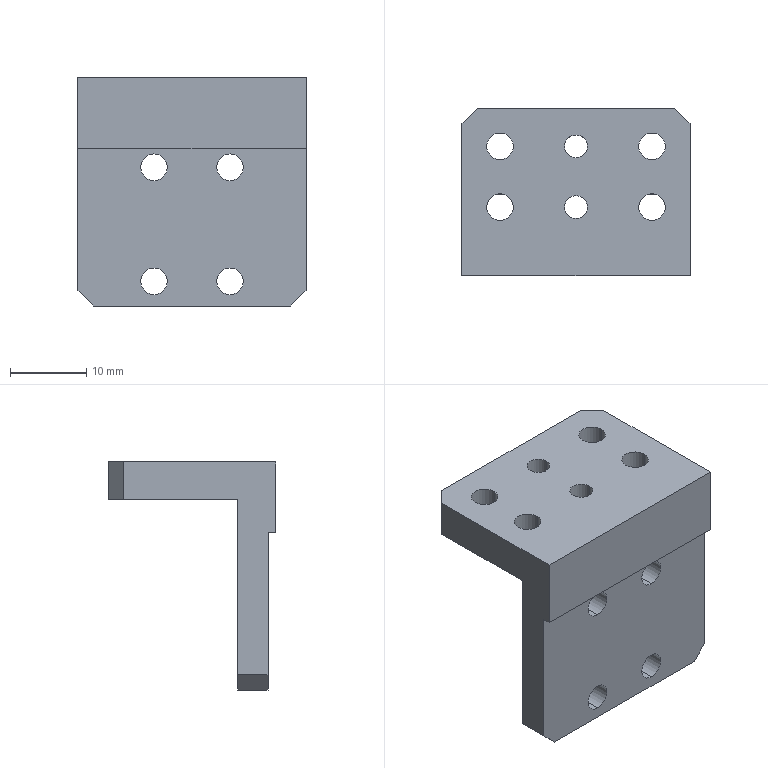Part | SolidWorks | features HoleWzd 3, ICE 2, Chamfer 1, Extrusion 1 | 1 solid | 34 faces | box 30 x 22 x 30 mm | volume 5974 mm3 | cylinder 20 | plane 14 | commonest cylinder face diameters 3.5 x16 3 x4
STEP:
#1=CARTESIAN_POINT('',(1.5,17.,15.));
#2=VERTEX_POINT('',#1);
#3=CARTESIAN_POINT('',(-1.5,17.,15.));
#4=VERTEX_POINT('',#3);
#5=CARTESIAN_POINT('',(0.,17.,15.));
#6=DIRECTION('',(0.,0.,-1.));
#7=DIRECTION('',(-1.,0.,0.));
#8=AXIS2_PLACEMENT_3D('',#5,#6,#7);
#9=CIRCLE('',#8,1.5);
#10=EDGE_CURVE('',#2,#4,#9,.T.);
#11=ORIENTED_EDGE('',*,*,#10,.F.);
#12=CARTESIAN_POINT('',(1.5,17.,10.));
#13=VERTEX_POINT('',#12);
#14=CARTESIAN_POINT('',(1.5,17.,10.));
#15=DIRECTION('',(0.,0.,-1.));
#16=VECTOR('',#15,1000.);
#17=LINE('',#14,#16);
#18=EDGE_CURVE('',#2,#13,#17,.T.);
#19=ORIENTED_EDGE('',*,*,#18,.T.);
#20=CARTESIAN_POINT('',(-1.5,17.,10.));
#21=VERTEX_POINT('',#20);
#22=CARTESIAN_POINT('',(0.,17.,10.));
#23=DIRECTION('',(0.,0.,-1.));
#24=DIRECTION('',(-1.,0.,0.));
#25=AXIS2_PLACEMENT_3D('',#22,#23,#24);
#26=CIRCLE('',#25,1.5);
#27=EDGE_CURVE('',#13,#21,#26,.T.);
#28=ORIENTED_EDGE('',*,*,#27,.T.);
#29=CARTESIAN_POINT('',(-1.5,17.,10.));
#30=DIRECTION('',(0.,0.,-1.));
#31=VECTOR('',#30,1000.);
#32=LINE('',#29,#31);
#33=EDGE_CURVE('',#4,#21,#32,.T.);
#34=ORIENTED_EDGE('',*,*,#33,.F.);
#35=EDGE_LOOP('',(#11,#19,#28,#34));
#36=FACE_OUTER_BOUND('',#35,.T.);
#37=CARTESIAN_POINT('',(0.,17.,10.));
#38=DIRECTION('',(0.,0.,-1.));
#39=DIRECTION('',(-1.,0.,0.));
#40=AXIS2_PLACEMENT_3D('',#37,#38,#39);
#41=CYLINDRICAL_SURFACE('',#40,1.5);
#42=ADVANCED_FACE('',(#36),#41,.F.);
#43=CARTESIAN_POINT('',(1.5,9.,15.));
#44=VERTEX_POINT('',#43);
#45=CARTESIAN_POINT('',(-1.5,9.,15.));
#46=VERTEX_POINT('',#45);
#47=CARTESIAN_POINT('',(0.,9.,15.));
#48=DIRECTION('',(0.,0.,-1.));
#49=DIRECTION('',(-1.,0.,0.));
#50=AXIS2_PLACEMENT_3D('',#47,#48,#49);
#51=CIRCLE('',#50,1.5);
#52=EDGE_CURVE('',#44,#46,#51,.T.);
#53=ORIENTED_EDGE('',*,*,#52,.F.);
#54=CARTESIAN_POINT('',(1.5,9.,10.));
#55=VERTEX_POINT('',#54);
#56=CARTESIAN_POINT('',(1.5,9.,10.));
#57=DIRECTION('',(0.,0.,-1.));
#58=VECTOR('',#57,1000.);
#59=LINE('',#56,#58);
#60=EDGE_CURVE('',#44,#55,#59,.T.);
#61=ORIENTED_EDGE('',*,*,#60,.T.);
#62=CARTESIAN_POINT('',(-1.5,9.,10.));
#63=VERTEX_POINT('',#62);
#64=CARTESIAN_POINT('',(0.,9.,10.));
#65=DIRECTION('',(0.,0.,-1.));
#66=DIRECTION('',(-1.,0.,0.));
#67=AXIS2_PLACEMENT_3D('',#64,#65,#66);
#68=CIRCLE('',#67,1.5);
#69=EDGE_CURVE('',#55,#63,#68,.T.);
#70=ORIENTED_EDGE('',*,*,#69,.T.);
#71=CARTESIAN_POINT('',(-1.5,9.,10.));
#72=DIRECTION('',(0.,0.,-1.));
#73=VECTOR('',#72,1000.);
#74=LINE('',#71,#73);
#75=EDGE_CURVE('',#46,#63,#74,.T.);
#76=ORIENTED_EDGE('',*,*,#75,.F.);
#77=EDGE_LOOP('',(#53,#61,#70,#76));
#78=FACE_OUTER_BOUND('',#77,.T.);
#79=CARTESIAN_POINT('',(0.,9.,10.));
#80=DIRECTION('',(0.,0.,-1.));
#81=DIRECTION('',(-1.,0.,0.));
#82=AXIS2_PLACEMENT_3D('',#79,#80,#81);
#83=CYLINDRICAL_SURFACE('',#82,1.5);
#84=ADVANCED_FACE('',(#78),#83,.F.);
#85=CARTESIAN_POINT('',(11.75,17.,15.));
#86=VERTEX_POINT('',#85);
#87=CARTESIAN_POINT('',(8.25,17.,15.));
#88=VERTEX_POINT('',#87);
#89=CARTESIAN_POINT('',(10.,17.,15.));
#90=DIRECTION('',(0.,0.,-1.));
#91=DIRECTION('',(-1.,0.,0.));
#92=AXIS2_PLACEMENT_3D('',#89,#90,#91);
#93=CIRCLE('',#92,1.75);
#94=EDGE_CURVE('',#86,#88,#93,.T.);
#95=ORIENTED_EDGE('',*,*,#94,.F.);
#96=CARTESIAN_POINT('',(11.75,17.,10.));
#97=VERTEX_POINT('',#96);
#98=CARTESIAN_POINT('',(11.75,17.,10.));
#99=DIRECTION('',(0.,0.,-1.));
#100=VECTOR('',#99,1000.);
#101=LINE('',#98,#100);
#102=EDGE_CURVE('',#86,#97,#101,.T.);
#103=ORIENTED_EDGE('',*,*,#102,.T.);
#104=CARTESIAN_POINT('',(8.25,17.,10.));
#105=VERTEX_POINT('',#104);
#106=CARTESIAN_POINT('',(10.,17.,10.));
#107=DIRECTION('',(0.,0.,-1.));
#108=DIRECTION('',(-1.,0.,0.));
#109=AXIS2_PLACEMENT_3D('',#106,#107,#108);
#110=CIRCLE('',#109,1.75);
#111=EDGE_CURVE('',#97,#105,#110,.T.);
#112=ORIENTED_EDGE('',*,*,#111,.T.);
#113=CARTESIAN_POINT('',(8.25,17.,10.));
#114=DIRECTION('',(0.,0.,-1.));
#115=VECTOR('',#114,1000.);
#116=LINE('',#113,#115);
#117=EDGE_CURVE('',#88,#105,#116,.T.);
#118=ORIENTED_EDGE('',*,*,#117,.F.);
#119=EDGE_LOOP('',(#95,#103,#112,#118));
#120=FACE_OUTER_BOUND('',#119,.T.);
#121=CARTESIAN_POINT('',(10.,17.,10.));
#122=DIRECTION('',(0.,0.,-1.));
#123=DIRECTION('',(-1.,0.,0.));
#124=AXIS2_PLACEMENT_3D('',#121,#122,#123);
#125=CYLINDRICAL_SURFACE('',#124,1.75);
#126=ADVANCED_FACE('',(#120),#125,.F.);
#127=CARTESIAN_POINT('',(-8.25,17.,15.));
#128=VERTEX_POINT('',#127);
#129=CARTESIAN_POINT('',(-11.75,17.,15.));
#130=VERTEX_POINT('',#129);
#131=CARTESIAN_POINT('',(-10.,17.,15.));
#132=DIRECTION('',(0.,0.,-1.));
#133=DIRECTION('',(-1.,0.,0.));
#134=AXIS2_PLACEMENT_3D('',#131,#132,#133);
#135=CIRCLE('',#134,1.75);
#136=EDGE_CURVE('',#128,#130,#135,.T.);
#137=ORIENTED_EDGE('',*,*,#136,.F.);
#138=CARTESIAN_POINT('',(-8.25,17.,10.));
#139=VERTEX_POINT('',#138);
#140=CARTESIAN_POINT('',(-8.25,17.,10.));
#141=DIRECTION('',(0.,0.,-1.));
#142=VECTOR('',#141,1000.);
#143=LINE('',#140,#142);
#144=EDGE_CURVE('',#128,#139,#143,.T.);
#145=ORIENTED_EDGE('',*,*,#144,.T.);
#146=CARTESIAN_POINT('',(-11.75,17.,10.));
#147=VERTEX_POINT('',#146);
#148=CARTESIAN_POINT('',(-10.,17.,10.));
#149=DIRECTION('',(0.,0.,-1.));
#150=DIRECTION('',(-1.,0.,0.));
#151=AXIS2_PLACEMENT_3D('',#148,#149,#150);
#152=CIRCLE('',#151,1.75);
#153=EDGE_CURVE('',#139,#147,#152,.T.);
#154=ORIENTED_EDGE('',*,*,#153,.T.);
#155=CARTESIAN_POINT('',(-11.75,17.,10.));
#156=DIRECTION('',(0.,0.,-1.));
#157=VECTOR('',#156,1000.);
#158=LINE('',#155,#157);
#159=EDGE_CURVE('',#130,#147,#158,.T.);
#160=ORIENTED_EDGE('',*,*,#159,.F.);
#161=EDGE_LOOP('',(#137,#145,#154,#160));
#162=FACE_OUTER_BOUND('',#161,.T.);
#163=CARTESIAN_POINT('',(-10.,17.,10.));
#164=DIRECTION('',(0.,0.,-1.));
#165=DIRECTION('',(-1.,0.,0.));
#166=AXIS2_PLACEMENT_3D('',#163,#164,#165);
#167=CYLINDRICAL_SURFACE('',#166,1.75);
#168=ADVANCED_FACE('',(#162),#167,.F.);
#169=CARTESIAN_POINT('',(11.75,9.,15.));
#170=VERTEX_POINT('',#169);
#171=CARTESIAN_POINT('',(8.25,9.,15.));
#172=VERTEX_POINT('',#171);
#173=CARTESIAN_POINT('',(10.,9.,15.));
#174=DIRECTION('',(0.,0.,-1.));
#175=DIRECTION('',(-1.,0.,0.));
#176=AXIS2_PLACEMENT_3D('',#173,#174,#175);
#177=CIRCLE('',#176,1.75);
#178=EDGE_CURVE('',#170,#172,#177,.T.);
#179=ORIENTED_EDGE('',*,*,#178,.F.);
#180=CARTESIAN_POINT('',(11.75,9.,10.));
#181=VERTEX_POINT('',#180);
#182=CARTESIAN_POINT('',(11.75,9.,10.));
#183=DIRECTION('',(0.,0.,-1.));
#184=VECTOR('',#183,1000.);
#185=LINE('',#182,#184);
#186=EDGE_CURVE('',#170,#181,#185,.T.);
#187=ORIENTED_EDGE('',*,*,#186,.T.);
#188=CARTESIAN_POINT('',(8.25,9.,10.));
#189=VERTEX_POINT('',#188);
#190=CARTESIAN_POINT('',(10.,9.,10.));
#191=DIRECTION('',(0.,0.,-1.));
#192=DIRECTION('',(-1.,0.,0.));
#193=AXIS2_PLACEMENT_3D('',#190,#191,#192);
#194=CIRCLE('',#193,1.75);
#195=EDGE_CURVE('',#181,#189,#194,.T.);
#196=ORIENTED_EDGE('',*,*,#195,.T.);
#197=CARTESIAN_POINT('',(8.25,9.,10.));
#198=DIRECTION('',(0.,0.,-1.));
#199=VECTOR('',#198,1000.);
#200=LINE('',#197,#199);
#201=EDGE_CURVE('',#172,#189,#200,.T.);
#202=ORIENTED_EDGE('',*,*,#201,.F.);
#203=EDGE_LOOP('',(#179,#187,#196,#202));
#204=FACE_OUTER_BOUND('',#203,.T.);
#205=CARTESIAN_POINT('',(10.,9.,10.));
#206=DIRECTION('',(0.,0.,-1.));
#207=DIRECTION('',(-1.,0.,0.));
#208=AXIS2_PLACEMENT_3D('',#205,#206,#207);
#209=CYLINDRICAL_SURFACE('',#208,1.75);
#210=ADVANCED_FACE('',(#204),#209,.F.);
#211=CARTESIAN_POINT('',(-8.25,9.,15.));
#212=VERTEX_POINT('',#211);
#213=CARTESIAN_POINT('',(-11.75,9.,15.));
#214=VERTEX_POINT('',#213);
#215=CARTESIAN_POINT('',(-10.,9.,15.));
#216=DIRECTION('',(0.,0.,-1.));
#217=DIRECTION('',(-1.,0.,0.));
#218=AXIS2_PLACEMENT_3D('',#215,#216,#217);
#219=CIRCLE('',#218,1.75);
#220=EDGE_CURVE('',#212,#214,#219,.T.);
#221=ORIENTED_EDGE('',*,*,#220,.F.);
#222=CARTESIAN_POINT('',(-8.25,9.,10.));
#223=VERTEX_POINT('',#222);
#224=CARTESIAN_POINT('',(-8.25,9.,10.));
#225=DIRECTION('',(0.,0.,-1.));
#226=VECTOR('',#225,1000.);
#227=LINE('',#224,#226);
#228=EDGE_CURVE('',#212,#223,#227,.T.);
#229=ORIENTED_EDGE('',*,*,#228,.T.);
#230=CARTESIAN_POINT('',(-11.75,9.,10.));
#231=VERTEX_POINT('',#230);
#232=CARTESIAN_POINT('',(-10.,9.,10.));
#233=DIRECTION('',(0.,0.,-1.));
#234=DIRECTION('',(-1.,0.,0.));
#235=AXIS2_PLACEMENT_3D('',#232,#233,#234);
#236=CIRCLE('',#235,1.75);
#237=EDGE_CURVE('',#223,#231,#236,.T.);
#238=ORIENTED_EDGE('',*,*,#237,.T.);
#239=CARTESIAN_POINT('',(-11.75,9.,10.));
#240=DIRECTION('',(0.,0.,-1.));
#241=VECTOR('',#240,1000.);
#242=LINE('',#239,#241);
#243=EDGE_CURVE('',#214,#231,#242,.T.);
#244=ORIENTED_EDGE('',*,*,#243,.F.);
#245=EDGE_LOOP('',(#221,#229,#238,#244));
#246=FACE_OUTER_BOUND('',#245,.T.);
#247=CARTESIAN_POINT('',(-10.,9.,10.));
#248=DIRECTION('',(0.,0.,-1.));
#249=DIRECTION('',(-1.,0.,0.));
#250=AXIS2_PLACEMENT_3D('',#247,#248,#249);
#251=CYLINDRICAL_SURFACE('',#250,1.75);
#252=ADVANCED_FACE('',(#246),#251,.F.);
#253=CARTESIAN_POINT('',(-5.,1.,-10.));
#254=VERTEX_POINT('',#253);
#255=CARTESIAN_POINT('',(-5.,1.,-13.5));
#256=VERTEX_POINT('',#255);
#257=CARTESIAN_POINT('',(-5.,1.,-11.75));
#258=DIRECTION('',(0.,-1.,0.));
#259=DIRECTION('',(0.,0.,1.));
#260=AXIS2_PLACEMENT_3D('',#257,#258,#259);
#261=CIRCLE('',#260,1.75);
#262=EDGE_CURVE('',#254,#256,#261,.T.);
#263=ORIENTED_EDGE('',*,*,#262,.T.);
#264=CARTESIAN_POINT('',(-5.,5.,-13.5));
#265=VERTEX_POINT('',#264);
#266=CARTESIAN_POINT('',(-5.,5.,-13.5));
#267=DIRECTION('',(0.,1.,0.));
#268=VECTOR('',#267,1000.);
#269=LINE('',#266,#268);
#270=EDGE_CURVE('',#256,#265,#269,.T.);
#271=ORIENTED_EDGE('',*,*,#270,.T.);
#272=CARTESIAN_POINT('',(-5.,5.,-10.));
#273=VERTEX_POINT('',#272);
#274=CARTESIAN_POINT('',(-5.,5.,-11.75));
#275=DIRECTION('',(0.,1.,0.));
#276=DIRECTION('',(0.,0.,1.));
#277=AXIS2_PLACEMENT_3D('',#274,#275,#276);
#278=CIRCLE('',#277,1.75);
#279=EDGE_CURVE('',#265,#273,#278,.T.);
#280=ORIENTED_EDGE('',*,*,#279,.T.);
#281=CARTESIAN_POINT('',(-5.,5.,-10.));
#282=DIRECTION('',(0.,1.,0.));
#283=VECTOR('',#282,1000.);
#284=LINE('',#281,#283);
#285=EDGE_CURVE('',#254,#273,#284,.T.);
#286=ORIENTED_EDGE('',*,*,#285,.F.);
#287=EDGE_LOOP('',(#263,#271,#280,#286));
#288=FACE_OUTER_BOUND('',#287,.T.);
#289=CARTESIAN_POINT('',(-5.,5.,-11.75));
#290=DIRECTION('',(0.,1.,0.));
#291=DIRECTION('',(0.,0.,1.));
#292=AXIS2_PLACEMENT_3D('',#289,#290,#291);
#293=CYLINDRICAL_SURFACE('',#292,1.75);
#294=ADVANCED_FACE('',(#288),#293,.F.);
#295=CARTESIAN_POINT('',(5.,1.,-10.));
#296=VERTEX_POINT('',#295);
#297=CARTESIAN_POINT('',(5.,1.,-13.5));
#298=VERTEX_POINT('',#297);
#299=CARTESIAN_POINT('',(5.,1.,-11.75));
#300=DIRECTION('',(0.,-1.,0.));
#301=DIRECTION('',(0.,0.,1.));
#302=AXIS2_PLACEMENT_3D('',#299,#300,#301);
#303=CIRCLE('',#302,1.75);
#304=EDGE_CURVE('',#296,#298,#303,.T.);
#305=ORIENTED_EDGE('',*,*,#304,.T.);
#306=CARTESIAN_POINT('',(5.,5.,-13.5));
#307=VERTEX_POINT('',#306);
#308=CARTESIAN_POINT('',(5.,5.,-13.5));
#309=DIRECTION('',(0.,1.,0.));
#310=VECTOR('',#309,1000.);
#311=LINE('',#308,#310);
#312=EDGE_CURVE('',#298,#307,#311,.T.);
#313=ORIENTED_EDGE('',*,*,#312,.T.);
#314=CARTESIAN_POINT('',(5.,5.,-10.));
#315=VERTEX_POINT('',#314);
#316=CARTESIAN_POINT('',(5.,5.,-11.75));
#317=DIRECTION('',(0.,1.,0.));
#318=DIRECTION('',(0.,0.,1.));
#319=AXIS2_PLACEMENT_3D('',#316,#317,#318);
#320=CIRCLE('',#319,1.75);
#321=EDGE_CURVE('',#307,#315,#320,.T.);
#322=ORIENTED_EDGE('',*,*,#321,.T.);
#323=CARTESIAN_POINT('',(5.,5.,-10.));
#324=DIRECTION('',(0.,1.,0.));
#325=VECTOR('',#324,1000.);
#326=LINE('',#323,#325);
#327=EDGE_CURVE('',#296,#315,#326,.T.);
#328=ORIENTED_EDGE('',*,*,#327,.F.);
#329=EDGE_LOOP('',(#305,#313,#322,#328));
#330=FACE_OUTER_BOUND('',#329,.T.);
#331=CARTESIAN_POINT('',(5.,5.,-11.75));
#332=DIRECTION('',(0.,1.,0.));
#333=DIRECTION('',(0.,0.,1.));
#334=AXIS2_PLACEMENT_3D('',#331,#332,#333);
#335=CYLINDRICAL_SURFACE('',#334,1.75);
#336=ADVANCED_FACE('',(#330),#335,.F.);
#337=CARTESIAN_POINT('',(5.,1.,5.));
#338=VERTEX_POINT('',#337);
#339=CARTESIAN_POINT('',(5.,1.,1.5));
#340=VERTEX_POINT('',#339);
#341=CARTESIAN_POINT('',(5.,1.,3.25));
#342=DIRECTION('',(0.,-1.,0.));
#343=DIRECTION('',(0.,0.,1.));
#344=AXIS2_PLACEMENT_3D('',#341,#342,#343);
#345=CIRCLE('',#344,1.75);
#346=EDGE_CURVE('',#338,#340,#345,.T.);
#347=ORIENTED_EDGE('',*,*,#346,.T.);
#348=CARTESIAN_POINT('',(5.,5.,1.5));
#349=VERTEX_POINT('',#348);
#350=CARTESIAN_POINT('',(5.,5.,1.5));
#351=DIRECTION('',(0.,1.,0.));
#352=VECTOR('',#351,1000.);
#353=LINE('',#350,#352);
#354=EDGE_CURVE('',#340,#349,#353,.T.);
#355=ORIENTED_EDGE('',*,*,#354,.T.);
#356=CARTESIAN_POINT('',(5.,5.,5.));
#357=VERTEX_POINT('',#356);
#358=CARTESIAN_POINT('',(5.,5.,3.25));
#359=DIRECTION('',(0.,1.,0.));
#360=DIRECTION('',(0.,0.,1.));
#361=AXIS2_PLACEMENT_3D('',#358,#359,#360);
#362=CIRCLE('',#361,1.75);
#363=EDGE_CURVE('',#349,#357,#362,.T.);
#364=ORIENTED_EDGE('',*,*,#363,.T.);
#365=CARTESIAN_POINT('',(5.,5.,5.));
#366=DIRECTION('',(0.,1.,0.));
#367=VECTOR('',#366,1000.);
#368=LINE('',#365,#367);
#369=EDGE_CURVE('',#338,#357,#368,.T.);
#370=ORIENTED_EDGE('',*,*,#369,.F.);
#371=EDGE_LOOP('',(#347,#355,#364,#370));
#372=FACE_OUTER_BOUND('',#371,.T.);
#373=CARTESIAN_POINT('',(5.,5.,3.25));
#374=DIRECTION('',(0.,1.,0.));
#375=DIRECTION('',(0.,0.,1.));
#376=AXIS2_PLACEMENT_3D('',#373,#374,#375);
#377=CYLINDRICAL_SURFACE('',#376,1.75);
#378=ADVANCED_FACE('',(#372),#377,.F.);
#379=CARTESIAN_POINT('',(-5.,1.,5.));
#380=VERTEX_POINT('',#379);
#381=CARTESIAN_POINT('',(-5.,1.,1.5));
#382=VERTEX_POINT('',#381);
#383=CARTESIAN_POINT('',(-5.,1.,3.25));
#384=DIRECTION('',(0.,-1.,0.));
#385=DIRECTION('',(0.,0.,1.));
#386=AXIS2_PLACEMENT_3D('',#383,#384,#385);
#387=CIRCLE('',#386,1.75);
#388=EDGE_CURVE('',#380,#382,#387,.T.);
#389=ORIENTED_EDGE('',*,*,#388,.T.);
#390=CARTESIAN_POINT('',(-5.,5.,1.5));
#391=VERTEX_POINT('',#390);
#392=CARTESIAN_POINT('',(-5.,5.,1.5));
#393=DIRECTION('',(0.,1.,0.));
#394=VECTOR('',#393,1000.);
#395=LINE('',#392,#394);
#396=EDGE_CURVE('',#382,#391,#395,.T.);
#397=ORIENTED_EDGE('',*,*,#396,.T.);
#398=CARTESIAN_POINT('',(-5.,5.,5.));
#399=VERTEX_POINT('',#398);
#400=CARTESIAN_POINT('',(-5.,5.,3.25));
#401=DIRECTION('',(0.,1.,0.));
#402=DIRECTION('',(0.,0.,1.));
#403=AXIS2_PLACEMENT_3D('',#400,#401,#402);
#404=CIRCLE('',#403,1.75);
#405=EDGE_CURVE('',#391,#399,#404,.T.);
#406=ORIENTED_EDGE('',*,*,#405,.T.);
#407=CARTESIAN_POINT('',(-5.,5.,5.));
#408=DIRECTION('',(0.,1.,0.));
#409=VECTOR('',#408,1000.);
#410=LINE('',#407,#409);
#411=EDGE_CURVE('',#380,#399,#410,.T.);
#412=ORIENTED_EDGE('',*,*,#411,.F.);
#413=EDGE_LOOP('',(#389,#397,#406,#412));
#414=FACE_OUTER_BOUND('',#413,.T.);
#415=CARTESIAN_POINT('',(-5.,5.,3.25));
#416=DIRECTION('',(0.,1.,0.));
#417=DIRECTION('',(0.,0.,1.));
#418=AXIS2_PLACEMENT_3D('',#415,#416,#417);
#419=CYLINDRICAL_SURFACE('',#418,1.75);
#420=ADVANCED_FACE('',(#414),#419,.F.);
#421=CARTESIAN_POINT('',(15.,1.,5.75));
#422=VERTEX_POINT('',#421);
#423=CARTESIAN_POINT('',(15.,1.,-13.));
#424=VERTEX_POINT('',#423);
#425=CARTESIAN_POINT('',(15.,1.,-15.));
#426=DIRECTION('',(0.,0.,-1.));
#427=VECTOR('',#426,1000.);
#428=LINE('',#425,#427);
#429=EDGE_CURVE('',#422,#424,#428,.T.);
#430=ORIENTED_EDGE('',*,*,#429,.T.);
#431=CARTESIAN_POINT('',(15.,5.,-13.));
#432=VERTEX_POINT('',#431);
#433=CARTESIAN_POINT('',(15.,5.,-13.));
#434=DIRECTION('',(0.,1.,0.));
#435=VECTOR('',#434,1000.);
#436=LINE('',#433,#435);
#437=EDGE_CURVE('',#424,#432,#436,.T.);
#438=ORIENTED_EDGE('',*,*,#437,.T.);
#439=CARTESIAN_POINT('',(15.,5.,10.));
#440=VERTEX_POINT('',#439);
#441=CARTESIAN_POINT('',(15.,5.,-15.));
#442=DIRECTION('',(0.,0.,-1.));
#443=VECTOR('',#442,1000.);
#444=LINE('',#441,#443);
#445=EDGE_CURVE('',#440,#432,#444,.T.);
#446=ORIENTED_EDGE('',*,*,#445,.F.);
#447=CARTESIAN_POINT('',(15.,20.,10.));
#448=VERTEX_POINT('',#447);
#449=CARTESIAN_POINT('',(15.,22.,10.));
#450=DIRECTION('',(0.,-1.,0.));
#451=VECTOR('',#450,1000.);
#452=LINE('',#449,#451);
#453=EDGE_CURVE('',#448,#440,#452,.T.);
#454=ORIENTED_EDGE('',*,*,#453,.F.);
#455=CARTESIAN_POINT('',(15.,20.,15.));
#456=VERTEX_POINT('',#455);
#457=CARTESIAN_POINT('',(15.,20.,-15.));
#458=DIRECTION('',(0.,0.,1.));
#459=VECTOR('',#458,1000.);
#460=LINE('',#457,#459);
#461=EDGE_CURVE('',#448,#456,#460,.T.);
#462=ORIENTED_EDGE('',*,*,#461,.T.);
#463=CARTESIAN_POINT('',(15.,0.,15.));
#464=VERTEX_POINT('',#463);
#465=CARTESIAN_POINT('',(15.,5.,15.));
#466=DIRECTION('',(0.,-1.,0.));
#467=VECTOR('',#466,1000.);
#468=LINE('',#465,#467);
#469=EDGE_CURVE('',#456,#464,#468,.T.);
#470=ORIENTED_EDGE('',*,*,#469,.T.);
#471=CARTESIAN_POINT('',(15.,0.,5.75));
#472=VERTEX_POINT('',#471);
#473=CARTESIAN_POINT('',(15.,0.,-15.));
#474=DIRECTION('',(0.,0.,-1.));
#475=VECTOR('',#474,1000.);
#476=LINE('',#473,#475);
#477=EDGE_CURVE('',#464,#472,#476,.T.);
#478=ORIENTED_EDGE('',*,*,#477,.T.);
#479=CARTESIAN_POINT('',(15.,0.,5.75));
#480=DIRECTION('',(0.,1.,0.));
#481=VECTOR('',#480,1000.);
#482=LINE('',#479,#481);
#483=EDGE_CURVE('',#472,#422,#482,.T.);
#484=ORIENTED_EDGE('',*,*,#483,.T.);
#485=EDGE_LOOP('',(#430,#438,#446,#454,#462,#470,#478,#484));
#486=FACE_OUTER_BOUND('',#485,.T.);
#487=CARTESIAN_POINT('',(15.,5.,-15.));
#488=DIRECTION('',(-1.,0.,0.));
#489=DIRECTION('',(0.,0.,1.));
#490=AXIS2_PLACEMENT_3D('',#487,#488,#489);
#491=PLANE('',#490);
#492=ADVANCED_FACE('',(#486),#491,.F.);
#493=CARTESIAN_POINT('',(13.,1.,-15.));
#494=VERTEX_POINT('',#493);
#495=CARTESIAN_POINT('',(-13.,1.,-15.));
#496=VERTEX_POINT('',#495);
#497=CARTESIAN_POINT('',(15.,1.,-15.));
#498=DIRECTION('',(-1.,0.,0.));
#499=VECTOR('',#498,1000.);
#500=LINE('',#497,#499);
#501=EDGE_CURVE('',#494,#496,#500,.T.);
#502=ORIENTED_EDGE('',*,*,#501,.T.);
#503=CARTESIAN_POINT('',(-13.,5.,-15.));
#504=VERTEX_POINT('',#503);
#505=CARTESIAN_POINT('',(-13.,5.,-15.));
#506=DIRECTION('',(0.,1.,0.));
#507=VECTOR('',#506,1000.);
#508=LINE('',#505,#507);
#509=EDGE_CURVE('',#496,#504,#508,.T.);
#510=ORIENTED_EDGE('',*,*,#509,.T.);
#511=CARTESIAN_POINT('',(13.,5.,-15.));
#512=VERTEX_POINT('',#511);
#513=CARTESIAN_POINT('',(-15.,5.,-15.));
#514=DIRECTION('',(-1.,0.,0.));
#515=VECTOR('',#514,1000.);
#516=LINE('',#513,#515);
#517=EDGE_CURVE('',#512,#504,#516,.T.);
#518=ORIENTED_EDGE('',*,*,#517,.F.);
#519=CARTESIAN_POINT('',(13.,5.,-15.));
#520=DIRECTION('',(0.,-1.,0.));
#521=VECTOR('',#520,1000.);
#522=LINE('',#519,#521);
#523=EDGE_CURVE('',#512,#494,#522,.T.);
#524=ORIENTED_EDGE('',*,*,#523,.T.);
#525=EDGE_LOOP('',(#502,#510,#518,#524));
#526=FACE_OUTER_BOUND('',#525,.T.);
#527=CARTESIAN_POINT('',(-15.,5.,-15.));
#528=DIRECTION('',(0.,0.,1.));
#529=DIRECTION('',(1.,0.,0.));
#530=AXIS2_PLACEMENT_3D('',#527,#528,#529);
#531=PLANE('',#530);
#532=ADVANCED_FACE('',(#526),#531,.F.);
#533=CARTESIAN_POINT('',(-15.,5.,-13.));
#534=VERTEX_POINT('',#533);
#535=CARTESIAN_POINT('',(-15.,5.,10.));
#536=VERTEX_POINT('',#535);
#537=CARTESIAN_POINT('',(-15.,5.,-15.));
#538=DIRECTION('',(0.,0.,1.));
#539=VECTOR('',#538,1000.);
#540=LINE('',#537,#539);
#541=EDGE_CURVE('',#534,#536,#540,.T.);
#542=ORIENTED_EDGE('',*,*,#541,.F.);
#543=CARTESIAN_POINT('',(-15.,1.,-13.));
#544=VERTEX_POINT('',#543);
#545=CARTESIAN_POINT('',(-15.,5.,-13.));
#546=DIRECTION('',(0.,-1.,0.));
#547=VECTOR('',#546,1000.);
#548=LINE('',#545,#547);
#549=EDGE_CURVE('',#534,#544,#548,.T.);
#550=ORIENTED_EDGE('',*,*,#549,.T.);
#551=CARTESIAN_POINT('',(-15.,1.,5.75));
#552=VERTEX_POINT('',#551);
#553=CARTESIAN_POINT('',(-15.,1.,-15.));
#554=DIRECTION('',(0.,0.,-1.));
#555=VECTOR('',#554,1000.);
#556=LINE('',#553,#555);
#557=EDGE_CURVE('',#552,#544,#556,.T.);
#558=ORIENTED_EDGE('',*,*,#557,.F.);
#559=CARTESIAN_POINT('',(-15.,0.,5.75));
#560=VERTEX_POINT('',#559);
#561=CARTESIAN_POINT('',(-15.,0.,5.75));
#562=DIRECTION('',(0.,1.,0.));
#563=VECTOR('',#562,1000.);
#564=LINE('',#561,#563);
#565=EDGE_CURVE('',#560,#552,#564,.T.);
#566=ORIENTED_EDGE('',*,*,#565,.F.);
#567=CARTESIAN_POINT('',(-15.,0.,15.));
#568=VERTEX_POINT('',#567);
#569=CARTESIAN_POINT('',(-15.,0.,-15.));
#570=DIRECTION('',(0.,0.,1.));
#571=VECTOR('',#570,1000.);
#572=LINE('',#569,#571);
#573=EDGE_CURVE('',#560,#568,#572,.T.);
#574=ORIENTED_EDGE('',*,*,#573,.T.);
#575=CARTESIAN_POINT('',(-15.,20.,15.));
#576=VERTEX_POINT('',#575);
#577=CARTESIAN_POINT('',(-15.,5.,15.));
#578=DIRECTION('',(0.,-1.,0.));
#579=VECTOR('',#578,1000.);
#580=LINE('',#577,#579);
#581=EDGE_CURVE('',#576,#568,#580,.T.);
#582=ORIENTED_EDGE('',*,*,#581,.F.);
#583=CARTESIAN_POINT('',(-15.,20.,10.));
#584=VERTEX_POINT('',#583);
#585=CARTESIAN_POINT('',(-15.,20.,-15.));
#586=DIRECTION('',(0.,0.,-1.));
#587=VECTOR('',#586,1000.);
#588=LINE('',#585,#587);
#589=EDGE_CURVE('',#576,#584,#588,.T.);
#590=ORIENTED_EDGE('',*,*,#589,.T.);
#591=CARTESIAN_POINT('',(-15.,22.,10.));
#592=DIRECTION('',(0.,-1.,0.));
#593=VECTOR('',#592,1000.);
#594=LINE('',#591,#593);
#595=EDGE_CURVE('',#584,#536,#594,.T.);
#596=ORIENTED_EDGE('',*,*,#595,.T.);
#597=EDGE_LOOP('',(#542,#550,#558,#566,#574,#582,#590,#596));
#598=FACE_OUTER_BOUND('',#597,.T.);
#599=CARTESIAN_POINT('',(-15.,5.,-15.));
#600=DIRECTION('',(1.,0.,0.));
#601=DIRECTION('',(0.,0.,-1.));
#602=AXIS2_PLACEMENT_3D('',#599,#600,#601);
#603=PLANE('',#602);
#604=ADVANCED_FACE('',(#598),#603,.F.);
#605=CARTESIAN_POINT('',(0.,17.,15.));
#606=DIRECTION('',(0.,0.,-1.));
#607=DIRECTION('',(-1.,0.,0.));
#608=AXIS2_PLACEMENT_3D('',#605,#606,#607);
#609=CIRCLE('',#608,1.5);
#610=EDGE_CURVE('',#4,#2,#609,.T.);
#611=ORIENTED_EDGE('',*,*,#610,.T.);
#612=ORIENTED_EDGE('',*,*,#10,.T.);
#613=EDGE_LOOP('',(#611,#612));
#614=FACE_BOUND('',#613,.T.);
#615=CARTESIAN_POINT('',(0.,9.,15.));
#616=DIRECTION('',(0.,0.,-1.));
#617=DIRECTION('',(-1.,0.,0.));
#618=AXIS2_PLACEMENT_3D('',#615,#616,#617);
#619=CIRCLE('',#618,1.5);
#620=EDGE_CURVE('',#46,#44,#619,.T.);
#621=ORIENTED_EDGE('',*,*,#620,.T.);
#622=ORIENTED_EDGE('',*,*,#52,.T.);
#623=EDGE_LOOP('',(#621,#622));
#624=FACE_BOUND('',#623,.T.);
#625=CARTESIAN_POINT('',(10.,17.,15.));
#626=DIRECTION('',(0.,0.,-1.));
#627=DIRECTION('',(-1.,0.,0.));
#628=AXIS2_PLACEMENT_3D('',#625,#626,#627);
#629=CIRCLE('',#628,1.75);
#630=EDGE_CURVE('',#88,#86,#629,.T.);
#631=ORIENTED_EDGE('',*,*,#630,.T.);
#632=ORIENTED_EDGE('',*,*,#94,.T.);
#633=EDGE_LOOP('',(#631,#632));
#634=FACE_BOUND('',#633,.T.);
#635=CARTESIAN_POINT('',(-10.,17.,15.));
#636=DIRECTION('',(0.,0.,-1.));
#637=DIRECTION('',(-1.,0.,0.));
#638=AXIS2_PLACEMENT_3D('',#635,#636,#637);
#639=CIRCLE('',#638,1.75);
#640=EDGE_CURVE('',#130,#128,#639,.T.);
#641=ORIENTED_EDGE('',*,*,#640,.T.);
#642=ORIENTED_EDGE('',*,*,#136,.T.);
#643=EDGE_LOOP('',(#641,#642));
#644=FACE_BOUND('',#643,.T.);
#645=CARTESIAN_POINT('',(10.,9.,15.));
#646=DIRECTION('',(0.,0.,-1.));
#647=DIRECTION('',(-1.,0.,0.));
#648=AXIS2_PLACEMENT_3D('',#645,#646,#647);
#649=CIRCLE('',#648,1.75);
#650=EDGE_CURVE('',#172,#170,#649,.T.);
#651=ORIENTED_EDGE('',*,*,#650,.T.);
#652=ORIENTED_EDGE('',*,*,#178,.T.);
#653=EDGE_LOOP('',(#651,#652));
#654=FACE_BOUND('',#653,.T.);
#655=CARTESIAN_POINT('',(-10.,9.,15.));
#656=DIRECTION('',(0.,0.,-1.));
#657=DIRECTION('',(-1.,0.,0.));
#658=AXIS2_PLACEMENT_3D('',#655,#656,#657);
#659=CIRCLE('',#658,1.75);
#660=EDGE_CURVE('',#214,#212,#659,.T.);
#661=ORIENTED_EDGE('',*,*,#660,.T.);
#662=ORIENTED_EDGE('',*,*,#220,.T.);
#663=EDGE_LOOP('',(#661,#662));
#664=FACE_BOUND('',#663,.T.);
#665=CARTESIAN_POINT('',(-13.,22.,15.));
#666=VERTEX_POINT('',#665);
#667=CARTESIAN_POINT('',(13.,22.,15.));
#668=VERTEX_POINT('',#667);
#669=CARTESIAN_POINT('',(-15.,22.,15.));
#670=DIRECTION('',(1.,0.,0.));
#671=VECTOR('',#670,1000.);
#672=LINE('',#669,#671);
#673=EDGE_CURVE('',#666,#668,#672,.T.);
#674=ORIENTED_EDGE('',*,*,#673,.F.);
#675=CARTESIAN_POINT('',(-13.,22.,15.));
#676=DIRECTION('',(-0.7071,-0.7071,0.));
#677=VECTOR('',#676,1000.);
#678=LINE('',#675,#677);
#679=EDGE_CURVE('',#666,#576,#678,.T.);
#680=ORIENTED_EDGE('',*,*,#679,.T.);
#681=ORIENTED_EDGE('',*,*,#581,.T.);
#682=CARTESIAN_POINT('',(-15.,0.,15.));
#683=DIRECTION('',(1.,0.,0.));
#684=VECTOR('',#683,1000.);
#685=LINE('',#682,#684);
#686=EDGE_CURVE('',#568,#464,#685,.T.);
#687=ORIENTED_EDGE('',*,*,#686,.T.);
#688=ORIENTED_EDGE('',*,*,#469,.F.);
#689=CARTESIAN_POINT('',(13.,22.,15.));
#690=DIRECTION('',(-0.7071,0.7071,0.));
#691=VECTOR('',#690,1000.);
#692=LINE('',#689,#691);
#693=EDGE_CURVE('',#456,#668,#692,.T.);
#694=ORIENTED_EDGE('',*,*,#693,.T.);
#695=EDGE_LOOP('',(#674,#680,#681,#687,#688,#694));
#696=FACE_OUTER_BOUND('',#695,.T.);
#697=CARTESIAN_POINT('',(-15.,5.,15.));
#698=DIRECTION('',(0.,0.,-1.));
#699=DIRECTION('',(-1.,0.,0.));
#700=AXIS2_PLACEMENT_3D('',#697,#698,#699);
#701=PLANE('',#700);
#702=ADVANCED_FACE('',(#614,#624,#634,#644,#654,#664,#696),#701,.F.);
#703=CARTESIAN_POINT('',(-5.,5.,-11.75));
#704=DIRECTION('',(0.,1.,0.));
#705=DIRECTION('',(0.,0.,1.));
#706=AXIS2_PLACEMENT_3D('',#703,#704,#705);
#707=CIRCLE('',#706,1.75);
#708=EDGE_CURVE('',#273,#265,#707,.T.);
#709=ORIENTED_EDGE('',*,*,#708,.F.);
#710=ORIENTED_EDGE('',*,*,#279,.F.);
#711=EDGE_LOOP('',(#709,#710));
#712=FACE_BOUND('',#711,.T.);
#713=CARTESIAN_POINT('',(5.,5.,-11.75));
#714=DIRECTION('',(0.,1.,0.));
#715=DIRECTION('',(0.,0.,1.));
#716=AXIS2_PLACEMENT_3D('',#713,#714,#715);
#717=CIRCLE('',#716,1.75);
#718=EDGE_CURVE('',#315,#307,#717,.T.);
#719=ORIENTED_EDGE('',*,*,#718,.F.);
#720=ORIENTED_EDGE('',*,*,#321,.F.);
#721=EDGE_LOOP('',(#719,#720));
#722=FACE_BOUND('',#721,.T.);
#723=CARTESIAN_POINT('',(5.,5.,3.25));
#724=DIRECTION('',(0.,1.,0.));
#725=DIRECTION('',(0.,0.,1.));
#726=AXIS2_PLACEMENT_3D('',#723,#724,#725);
#727=CIRCLE('',#726,1.75);
#728=EDGE_CURVE('',#357,#349,#727,.T.);
#729=ORIENTED_EDGE('',*,*,#728,.F.);
#730=ORIENTED_EDGE('',*,*,#363,.F.);
#731=EDGE_LOOP('',(#729,#730));
#732=FACE_BOUND('',#731,.T.);
#733=CARTESIAN_POINT('',(-5.,5.,3.25));
#734=DIRECTION('',(0.,1.,0.));
#735=DIRECTION('',(0.,0.,1.));
#736=AXIS2_PLACEMENT_3D('',#733,#734,#735);
#737=CIRCLE('',#736,1.75);
#738=EDGE_CURVE('',#399,#391,#737,.T.);
#739=ORIENTED_EDGE('',*,*,#738,.F.);
#740=ORIENTED_EDGE('',*,*,#405,.F.);
#741=EDGE_LOOP('',(#739,#740));
#742=FACE_BOUND('',#741,.T.);
#743=ORIENTED_EDGE('',*,*,#517,.T.);
#744=CARTESIAN_POINT('',(-14.,5.,-14.));
#745=DIRECTION('',(-0.7071,0.,0.7071));
#746=VECTOR('',#745,1000.);
#747=LINE('',#744,#746);
#748=EDGE_CURVE('',#504,#534,#747,.T.);
#749=ORIENTED_EDGE('',*,*,#748,.T.);
#750=ORIENTED_EDGE('',*,*,#541,.T.);
#751=CARTESIAN_POINT('',(-15.,5.,10.));
#752=DIRECTION('',(-1.,0.,0.));
#753=VECTOR('',#752,1000.);
#754=LINE('',#751,#753);
#755=EDGE_CURVE('',#440,#536,#754,.T.);
#756=ORIENTED_EDGE('',*,*,#755,.F.);
#757=ORIENTED_EDGE('',*,*,#445,.T.);
#758=CARTESIAN_POINT('',(14.,5.,-14.));
#759=DIRECTION('',(-0.7071,0.,-0.7071));
#760=VECTOR('',#759,1000.);
#761=LINE('',#758,#760);
#762=EDGE_CURVE('',#432,#512,#761,.T.);
#763=ORIENTED_EDGE('',*,*,#762,.T.);
#764=EDGE_LOOP('',(#743,#749,#750,#756,#757,#763));
#765=FACE_OUTER_BOUND('',#764,.T.);
#766=CARTESIAN_POINT('',(0.,5.,0.));
#767=DIRECTION('',(0.,1.,0.));
#768=DIRECTION('',(0.,0.,1.));
#769=AXIS2_PLACEMENT_3D('',#766,#767,#768);
#770=PLANE('',#769);
#771=ADVANCED_FACE('',(#712,#722,#732,#742,#765),#770,.T.);
#772=ORIENTED_EDGE('',*,*,#573,.F.);
#773=CARTESIAN_POINT('',(15.,0.,5.75));
#774=DIRECTION('',(-1.,0.,0.));
#775=VECTOR('',#774,1000.);
#776=LINE('',#773,#775);
#777=EDGE_CURVE('',#472,#560,#776,.T.);
#778=ORIENTED_EDGE('',*,*,#777,.F.);
#779=ORIENTED_EDGE('',*,*,#477,.F.);
#780=ORIENTED_EDGE('',*,*,#686,.F.);
#781=EDGE_LOOP('',(#772,#778,#779,#780));
#782=FACE_OUTER_BOUND('',#781,.T.);
#783=CARTESIAN_POINT('',(0.,0.,0.));
#784=DIRECTION('',(0.,1.,0.));
#785=DIRECTION('',(0.,0.,1.));
#786=AXIS2_PLACEMENT_3D('',#783,#784,#785);
#787=PLANE('',#786);
#788=ADVANCED_FACE('',(#782),#787,.F.);
#789=CARTESIAN_POINT('',(0.,17.,10.));
#790=DIRECTION('',(0.,0.,-1.));
#791=DIRECTION('',(-1.,0.,0.));
#792=AXIS2_PLACEMENT_3D('',#789,#790,#791);
#793=CIRCLE('',#792,1.5);
#794=EDGE_CURVE('',#21,#13,#793,.T.);
#795=ORIENTED_EDGE('',*,*,#794,.F.);
#796=ORIENTED_EDGE('',*,*,#27,.F.);
#797=EDGE_LOOP('',(#795,#796));
#798=FACE_BOUND('',#797,.T.);
#799=CARTESIAN_POINT('',(0.,9.,10.));
#800=DIRECTION('',(0.,0.,-1.));
#801=DIRECTION('',(-1.,0.,0.));
#802=AXIS2_PLACEMENT_3D('',#799,#800,#801);
#803=CIRCLE('',#802,1.5);
#804=EDGE_CURVE('',#63,#55,#803,.T.);
#805=ORIENTED_EDGE('',*,*,#804,.F.);
#806=ORIENTED_EDGE('',*,*,#69,.F.);
#807=EDGE_LOOP('',(#805,#806));
#808=FACE_BOUND('',#807,.T.);
#809=CARTESIAN_POINT('',(10.,17.,10.));
#810=DIRECTION('',(0.,0.,-1.));
#811=DIRECTION('',(-1.,0.,0.));
#812=AXIS2_PLACEMENT_3D('',#809,#810,#811);
#813=CIRCLE('',#812,1.75);
#814=EDGE_CURVE('',#105,#97,#813,.T.);
#815=ORIENTED_EDGE('',*,*,#814,.F.);
#816=ORIENTED_EDGE('',*,*,#111,.F.);
#817=EDGE_LOOP('',(#815,#816));
#818=FACE_BOUND('',#817,.T.);
#819=CARTESIAN_POINT('',(-10.,17.,10.));
#820=DIRECTION('',(0.,0.,-1.));
#821=DIRECTION('',(-1.,0.,0.));
#822=AXIS2_PLACEMENT_3D('',#819,#820,#821);
#823=CIRCLE('',#822,1.75);
#824=EDGE_CURVE('',#147,#139,#823,.T.);
#825=ORIENTED_EDGE('',*,*,#824,.F.);
#826=ORIENTED_EDGE('',*,*,#153,.F.);
#827=EDGE_LOOP('',(#825,#826));
#828=FACE_BOUND('',#827,.T.);
#829=CARTESIAN_POINT('',(10.,9.,10.));
#830=DIRECTION('',(0.,0.,-1.));
#831=DIRECTION('',(-1.,0.,0.));
#832=AXIS2_PLACEMENT_3D('',#829,#830,#831);
#833=CIRCLE('',#832,1.75);
#834=EDGE_CURVE('',#189,#181,#833,.T.);
#835=ORIENTED_EDGE('',*,*,#834,.F.);
#836=ORIENTED_EDGE('',*,*,#195,.F.);
#837=EDGE_LOOP('',(#835,#836));
#838=FACE_BOUND('',#837,.T.);
#839=CARTESIAN_POINT('',(-10.,9.,10.));
#840=DIRECTION('',(0.,0.,-1.));
#841=DIRECTION('',(-1.,0.,0.));
#842=AXIS2_PLACEMENT_3D('',#839,#840,#841);
#843=CIRCLE('',#842,1.75);
#844=EDGE_CURVE('',#231,#223,#843,.T.);
#845=ORIENTED_EDGE('',*,*,#844,.F.);
#846=ORIENTED_EDGE('',*,*,#237,.F.);
#847=EDGE_LOOP('',(#845,#846));
#848=FACE_BOUND('',#847,.T.);
#849=ORIENTED_EDGE('',*,*,#595,.F.);
#850=CARTESIAN_POINT('',(-13.,22.,10.));
#851=VERTEX_POINT('',#850);
#852=CARTESIAN_POINT('',(-13.,22.,10.));
#853=DIRECTION('',(0.7071,0.7071,0.));
#854=VECTOR('',#853,1000.);
#855=LINE('',#852,#854);
#856=EDGE_CURVE('',#584,#851,#855,.T.);
#857=ORIENTED_EDGE('',*,*,#856,.T.);
#858=CARTESIAN_POINT('',(13.,22.,10.));
#859=VERTEX_POINT('',#858);
#860=CARTESIAN_POINT('',(-15.,22.,10.));
#861=DIRECTION('',(-1.,0.,0.));
#862=VECTOR('',#861,1000.);
#863=LINE('',#860,#862);
#864=EDGE_CURVE('',#859,#851,#863,.T.);
#865=ORIENTED_EDGE('',*,*,#864,.F.);
#866=CARTESIAN_POINT('',(13.,22.,10.));
#867=DIRECTION('',(0.7071,-0.7071,0.));
#868=VECTOR('',#867,1000.);
#869=LINE('',#866,#868);
#870=EDGE_CURVE('',#859,#448,#869,.T.);
#871=ORIENTED_EDGE('',*,*,#870,.T.);
#872=ORIENTED_EDGE('',*,*,#453,.T.);
#873=ORIENTED_EDGE('',*,*,#755,.T.);
#874=EDGE_LOOP('',(#849,#857,#865,#871,#872,#873));
#875=FACE_OUTER_BOUND('',#874,.T.);
#876=CARTESIAN_POINT('',(-15.,22.,10.));
#877=DIRECTION('',(0.,0.,1.));
#878=DIRECTION('',(1.,0.,0.));
#879=AXIS2_PLACEMENT_3D('',#876,#877,#878);
#880=PLANE('',#879);
#881=ADVANCED_FACE('',(#798,#808,#818,#828,#838,#848,#875),#880,.F.);
#882=ORIENTED_EDGE('',*,*,#864,.T.);
#883=CARTESIAN_POINT('',(-13.,22.,0.));
#884=DIRECTION('',(0.,0.,1.));
#885=VECTOR('',#884,1000.);
#886=LINE('',#883,#885);
#887=EDGE_CURVE('',#851,#666,#886,.T.);
#888=ORIENTED_EDGE('',*,*,#887,.T.);
#889=ORIENTED_EDGE('',*,*,#673,.T.);
#890=CARTESIAN_POINT('',(13.,22.,0.));
#891=DIRECTION('',(0.,0.,-1.));
#892=VECTOR('',#891,1000.);
#893=LINE('',#890,#892);
#894=EDGE_CURVE('',#668,#859,#893,.T.);
#895=ORIENTED_EDGE('',*,*,#894,.T.);
#896=EDGE_LOOP('',(#882,#888,#889,#895));
#897=FACE_OUTER_BOUND('',#896,.T.);
#898=CARTESIAN_POINT('',(0.,22.,0.));
#899=DIRECTION('',(0.,-1.,0.));
#900=DIRECTION('',(0.,0.,-1.));
#901=AXIS2_PLACEMENT_3D('',#898,#899,#900);
#902=PLANE('',#901);
#903=ADVANCED_FACE('',(#897),#902,.F.);
#904=ORIENTED_EDGE('',*,*,#396,.F.);
#905=CARTESIAN_POINT('',(-5.,1.,3.25));
#906=DIRECTION('',(0.,-1.,0.));
#907=DIRECTION('',(0.,0.,1.));
#908=AXIS2_PLACEMENT_3D('',#905,#906,#907);
#909=CIRCLE('',#908,1.75);
#910=EDGE_CURVE('',#382,#380,#909,.T.);
#911=ORIENTED_EDGE('',*,*,#910,.T.);
#912=ORIENTED_EDGE('',*,*,#411,.T.);
#913=ORIENTED_EDGE('',*,*,#738,.T.);
#914=EDGE_LOOP('',(#904,#911,#912,#913));
#915=FACE_OUTER_BOUND('',#914,.T.);
#916=CARTESIAN_POINT('',(-5.,5.,3.25));
#917=DIRECTION('',(0.,1.,0.));
#918=DIRECTION('',(0.,0.,1.));
#919=AXIS2_PLACEMENT_3D('',#916,#917,#918);
#920=CYLINDRICAL_SURFACE('',#919,1.75);
#921=ADVANCED_FACE('',(#915),#920,.F.);
#922=ORIENTED_EDGE('',*,*,#354,.F.);
#923=CARTESIAN_POINT('',(5.,1.,3.25));
#924=DIRECTION('',(0.,-1.,0.));
#925=DIRECTION('',(0.,0.,1.));
#926=AXIS2_PLACEMENT_3D('',#923,#924,#925);
#927=CIRCLE('',#926,1.75);
#928=EDGE_CURVE('',#340,#338,#927,.T.);
#929=ORIENTED_EDGE('',*,*,#928,.T.);
#930=ORIENTED_EDGE('',*,*,#369,.T.);
#931=ORIENTED_EDGE('',*,*,#728,.T.);
#932=EDGE_LOOP('',(#922,#929,#930,#931));
#933=FACE_OUTER_BOUND('',#932,.T.);
#934=CARTESIAN_POINT('',(5.,5.,3.25));
#935=DIRECTION('',(0.,1.,0.));
#936=DIRECTION('',(0.,0.,1.));
#937=AXIS2_PLACEMENT_3D('',#934,#935,#936);
#938=CYLINDRICAL_SURFACE('',#937,1.75);
#939=ADVANCED_FACE('',(#933),#938,.F.);
#940=ORIENTED_EDGE('',*,*,#312,.F.);
#941=CARTESIAN_POINT('',(5.,1.,-11.75));
#942=DIRECTION('',(0.,-1.,0.));
#943=DIRECTION('',(0.,0.,1.));
#944=AXIS2_PLACEMENT_3D('',#941,#942,#943);
#945=CIRCLE('',#944,1.75);
#946=EDGE_CURVE('',#298,#296,#945,.T.);
#947=ORIENTED_EDGE('',*,*,#946,.T.);
#948=ORIENTED_EDGE('',*,*,#327,.T.);
#949=ORIENTED_EDGE('',*,*,#718,.T.);
#950=EDGE_LOOP('',(#940,#947,#948,#949));
#951=FACE_OUTER_BOUND('',#950,.T.);
#952=CARTESIAN_POINT('',(5.,5.,-11.75));
#953=DIRECTION('',(0.,1.,0.));
#954=DIRECTION('',(0.,0.,1.));
#955=AXIS2_PLACEMENT_3D('',#952,#953,#954);
#956=CYLINDRICAL_SURFACE('',#955,1.75);
#957=ADVANCED_FACE('',(#951),#956,.F.);
#958=ORIENTED_EDGE('',*,*,#270,.F.);
#959=CARTESIAN_POINT('',(-5.,1.,-11.75));
#960=DIRECTION('',(0.,-1.,0.));
#961=DIRECTION('',(0.,0.,1.));
#962=AXIS2_PLACEMENT_3D('',#959,#960,#961);
#963=CIRCLE('',#962,1.75);
#964=EDGE_CURVE('',#256,#254,#963,.T.);
#965=ORIENTED_EDGE('',*,*,#964,.T.);
#966=ORIENTED_EDGE('',*,*,#285,.T.);
#967=ORIENTED_EDGE('',*,*,#708,.T.);
#968=EDGE_LOOP('',(#958,#965,#966,#967));
#969=FACE_OUTER_BOUND('',#968,.T.);
#970=CARTESIAN_POINT('',(-5.,5.,-11.75));
#971=DIRECTION('',(0.,1.,0.));
#972=DIRECTION('',(0.,0.,1.));
#973=AXIS2_PLACEMENT_3D('',#970,#971,#972);
#974=CYLINDRICAL_SURFACE('',#973,1.75);
#975=ADVANCED_FACE('',(#969),#974,.F.);
#976=ORIENTED_EDGE('',*,*,#346,.F.);
#977=ORIENTED_EDGE('',*,*,#928,.F.);
#978=EDGE_LOOP('',(#976,#977));
#979=FACE_BOUND('',#978,.T.);
#980=ORIENTED_EDGE('',*,*,#262,.F.);
#981=ORIENTED_EDGE('',*,*,#964,.F.);
#982=EDGE_LOOP('',(#980,#981));
#983=FACE_BOUND('',#982,.T.);
#984=ORIENTED_EDGE('',*,*,#557,.T.);
#985=CARTESIAN_POINT('',(-15.,1.,-13.));
#986=DIRECTION('',(0.7071,0.,-0.7071));
#987=VECTOR('',#986,1000.);
#988=LINE('',#985,#987);
#989=EDGE_CURVE('',#544,#496,#988,.T.);
#990=ORIENTED_EDGE('',*,*,#989,.T.);
#991=ORIENTED_EDGE('',*,*,#501,.F.);
#992=CARTESIAN_POINT('',(13.,1.,-15.));
#993=DIRECTION('',(0.7071,0.,0.7071));
#994=VECTOR('',#993,1000.);
#995=LINE('',#992,#994);
#996=EDGE_CURVE('',#494,#424,#995,.T.);
#997=ORIENTED_EDGE('',*,*,#996,.T.);
#998=ORIENTED_EDGE('',*,*,#429,.F.);
#999=CARTESIAN_POINT('',(15.,1.,5.75));
#1000=DIRECTION('',(-1.,0.,0.));
#1001=VECTOR('',#1000,1000.);
#1002=LINE('',#999,#1001);
#1003=EDGE_CURVE('',#422,#552,#1002,.T.);
#1004=ORIENTED_EDGE('',*,*,#1003,.T.);
#1005=EDGE_LOOP('',(#984,#990,#991,#997,#998,#1004));
#1006=FACE_OUTER_BOUND('',#1005,.T.);
#1007=ORIENTED_EDGE('',*,*,#304,.F.);
#1008=ORIENTED_EDGE('',*,*,#946,.F.);
#1009=EDGE_LOOP('',(#1007,#1008));
#1010=FACE_BOUND('',#1009,.T.);
#1011=ORIENTED_EDGE('',*,*,#388,.F.);
#1012=ORIENTED_EDGE('',*,*,#910,.F.);
#1013=EDGE_LOOP('',(#1011,#1012));
#1014=FACE_BOUND('',#1013,.T.);
#1015=CARTESIAN_POINT('',(15.,1.,-15.));
#1016=DIRECTION('',(0.,1.,0.));
#1017=DIRECTION('',(0.,0.,1.));
#1018=AXIS2_PLACEMENT_3D('',#1015,#1016,#1017);
#1019=PLANE('',#1018);
#1020=ADVANCED_FACE('',(#979,#983,#1006,#1010,#1014),#1019,.F.);
#1021=ORIENTED_EDGE('',*,*,#565,.T.);
#1022=ORIENTED_EDGE('',*,*,#1003,.F.);
#1023=ORIENTED_EDGE('',*,*,#483,.F.);
#1024=ORIENTED_EDGE('',*,*,#777,.T.);
#1025=EDGE_LOOP('',(#1021,#1022,#1023,#1024));
#1026=FACE_OUTER_BOUND('',#1025,.T.);
#1027=CARTESIAN_POINT('',(15.,0.,5.75));
#1028=DIRECTION('',(0.,0.,1.));
#1029=DIRECTION('',(1.,0.,0.));
#1030=AXIS2_PLACEMENT_3D('',#1027,#1028,#1029);
#1031=PLANE('',#1030);
#1032=ADVANCED_FACE('',(#1026),#1031,.F.);
#1033=ORIENTED_EDGE('',*,*,#748,.F.);
#1034=ORIENTED_EDGE('',*,*,#509,.F.);
#1035=ORIENTED_EDGE('',*,*,#989,.F.);
#1036=ORIENTED_EDGE('',*,*,#549,.F.);
#1037=EDGE_LOOP('',(#1033,#1034,#1035,#1036));
#1038=FACE_OUTER_BOUND('',#1037,.T.);
#1039=CARTESIAN_POINT('',(-15.,5.,-13.));
#1040=DIRECTION('',(0.7071,0.,0.7071));
#1041=DIRECTION('',(0.,-1.,0.));
#1042=AXIS2_PLACEMENT_3D('',#1039,#1040,#1041);
#1043=PLANE('',#1042);
#1044=ADVANCED_FACE('',(#1038),#1043,.F.);
#1045=ORIENTED_EDGE('',*,*,#762,.F.);
#1046=ORIENTED_EDGE('',*,*,#437,.F.);
#1047=ORIENTED_EDGE('',*,*,#996,.F.);
#1048=ORIENTED_EDGE('',*,*,#523,.F.);
#1049=EDGE_LOOP('',(#1045,#1046,#1047,#1048));
#1050=FACE_OUTER_BOUND('',#1049,.T.);
#1051=CARTESIAN_POINT('',(13.,5.,-15.));
#1052=DIRECTION('',(-0.7071,0.,0.7071));
#1053=DIRECTION('',(0.,-1.,0.));
#1054=AXIS2_PLACEMENT_3D('',#1051,#1052,#1053);
#1055=PLANE('',#1054);
#1056=ADVANCED_FACE('',(#1050),#1055,.F.);
#1057=ORIENTED_EDGE('',*,*,#856,.F.);
#1058=ORIENTED_EDGE('',*,*,#589,.F.);
#1059=ORIENTED_EDGE('',*,*,#679,.F.);
#1060=ORIENTED_EDGE('',*,*,#887,.F.);
#1061=EDGE_LOOP('',(#1057,#1058,#1059,#1060));
#1062=FACE_OUTER_BOUND('',#1061,.T.);
#1063=CARTESIAN_POINT('',(-13.,22.,0.));
#1064=DIRECTION('',(0.7071,-0.7071,0.));
#1065=DIRECTION('',(0.,0.,1.));
#1066=AXIS2_PLACEMENT_3D('',#1063,#1064,#1065);
#1067=PLANE('',#1066);
#1068=ADVANCED_FACE('',(#1062),#1067,.F.);
#1069=ORIENTED_EDGE('',*,*,#693,.F.);
#1070=ORIENTED_EDGE('',*,*,#461,.F.);
#1071=ORIENTED_EDGE('',*,*,#870,.F.);
#1072=ORIENTED_EDGE('',*,*,#894,.F.);
#1073=EDGE_LOOP('',(#1069,#1070,#1071,#1072));
#1074=FACE_OUTER_BOUND('',#1073,.T.);
#1075=CARTESIAN_POINT('',(13.,22.,0.));
#1076=DIRECTION('',(-0.7071,-0.7071,0.));
#1077=DIRECTION('',(0.,0.,-1.));
#1078=AXIS2_PLACEMENT_3D('',#1075,#1076,#1077);
#1079=PLANE('',#1078);
#1080=ADVANCED_FACE('',(#1074),#1079,.F.);
#1081=ORIENTED_EDGE('',*,*,#228,.F.);
#1082=ORIENTED_EDGE('',*,*,#660,.F.);
#1083=ORIENTED_EDGE('',*,*,#243,.T.);
#1084=ORIENTED_EDGE('',*,*,#844,.T.);
#1085=EDGE_LOOP('',(#1081,#1082,#1083,#1084));
#1086=FACE_OUTER_BOUND('',#1085,.T.);
#1087=CARTESIAN_POINT('',(-10.,9.,10.));
#1088=DIRECTION('',(0.,0.,-1.));
#1089=DIRECTION('',(-1.,0.,0.));
#1090=AXIS2_PLACEMENT_3D('',#1087,#1088,#1089);
#1091=CYLINDRICAL_SURFACE('',#1090,1.75);
#1092=ADVANCED_FACE('',(#1086),#1091,.F.);
#1093=ORIENTED_EDGE('',*,*,#186,.F.);
#1094=ORIENTED_EDGE('',*,*,#650,.F.);
#1095=ORIENTED_EDGE('',*,*,#201,.T.);
#1096=ORIENTED_EDGE('',*,*,#834,.T.);
#1097=EDGE_LOOP('',(#1093,#1094,#1095,#1096));
#1098=FACE_OUTER_BOUND('',#1097,.T.);
#1099=CARTESIAN_POINT('',(10.,9.,10.));
#1100=DIRECTION('',(0.,0.,-1.));
#1101=DIRECTION('',(-1.,0.,0.));
#1102=AXIS2_PLACEMENT_3D('',#1099,#1100,#1101);
#1103=CYLINDRICAL_SURFACE('',#1102,1.75);
#1104=ADVANCED_FACE('',(#1098),#1103,.F.);
#1105=ORIENTED_EDGE('',*,*,#144,.F.);
#1106=ORIENTED_EDGE('',*,*,#640,.F.);
#1107=ORIENTED_EDGE('',*,*,#159,.T.);
#1108=ORIENTED_EDGE('',*,*,#824,.T.);
#1109=EDGE_LOOP('',(#1105,#1106,#1107,#1108));
#1110=FACE_OUTER_BOUND('',#1109,.T.);
#1111=CARTESIAN_POINT('',(-10.,17.,10.));
#1112=DIRECTION('',(0.,0.,-1.));
#1113=DIRECTION('',(-1.,0.,0.));
#1114=AXIS2_PLACEMENT_3D('',#1111,#1112,#1113);
#1115=CYLINDRICAL_SURFACE('',#1114,1.75);
#1116=ADVANCED_FACE('',(#1110),#1115,.F.);
#1117=ORIENTED_EDGE('',*,*,#102,.F.);
#1118=ORIENTED_EDGE('',*,*,#630,.F.);
#1119=ORIENTED_EDGE('',*,*,#117,.T.);
#1120=ORIENTED_EDGE('',*,*,#814,.T.);
#1121=EDGE_LOOP('',(#1117,#1118,#1119,#1120));
#1122=FACE_OUTER_BOUND('',#1121,.T.);
#1123=CARTESIAN_POINT('',(10.,17.,10.));
#1124=DIRECTION('',(0.,0.,-1.));
#1125=DIRECTION('',(-1.,0.,0.));
#1126=AXIS2_PLACEMENT_3D('',#1123,#1124,#1125);
#1127=CYLINDRICAL_SURFACE('',#1126,1.75);
#1128=ADVANCED_FACE('',(#1122),#1127,.F.);
#1129=ORIENTED_EDGE('',*,*,#60,.F.);
#1130=ORIENTED_EDGE('',*,*,#620,.F.);
#1131=ORIENTED_EDGE('',*,*,#75,.T.);
#1132=ORIENTED_EDGE('',*,*,#804,.T.);
#1133=EDGE_LOOP('',(#1129,#1130,#1131,#1132));
#1134=FACE_OUTER_BOUND('',#1133,.T.);
#1135=CARTESIAN_POINT('',(0.,9.,10.));
#1136=DIRECTION('',(0.,0.,-1.));
#1137=DIRECTION('',(-1.,0.,0.));
#1138=AXIS2_PLACEMENT_3D('',#1135,#1136,#1137);
#1139=CYLINDRICAL_SURFACE('',#1138,1.5);
#1140=ADVANCED_FACE('',(#1134),#1139,.F.);
#1141=ORIENTED_EDGE('',*,*,#18,.F.);
#1142=ORIENTED_EDGE('',*,*,#610,.F.);
#1143=ORIENTED_EDGE('',*,*,#33,.T.);
#1144=ORIENTED_EDGE('',*,*,#794,.T.);
#1145=EDGE_LOOP('',(#1141,#1142,#1143,#1144));
#1146=FACE_OUTER_BOUND('',#1145,.T.);
#1147=CARTESIAN_POINT('',(0.,17.,10.));
#1148=DIRECTION('',(0.,0.,-1.));
#1149=DIRECTION('',(-1.,0.,0.));
#1150=AXIS2_PLACEMENT_3D('',#1147,#1148,#1149);
#1151=CYLINDRICAL_SURFACE('',#1150,1.5);
#1152=ADVANCED_FACE('',(#1146),#1151,.F.);
#1153=CLOSED_SHELL('',(#42,#84,#126,#168,#210,#252,#294,#336,#378,#420,#492,#532,#604,#702,#771,#788,#881,#903,#921,#939,#957,#975,#1020,#1032,#1044,#1056,#1068,#1080,#1092,#1104,#1116,#1128,#1140,#1152));
#1154=MANIFOLD_SOLID_BREP('',#1153);
#1155=CARTESIAN_POINT('',(0.,0.,0.));
#1156=DIRECTION('',(0.,0.,1.));
#1157=DIRECTION('',(1.,0.,0.));
#1158=AXIS2_PLACEMENT_3D('',#1155,#1156,#1157);
#1159=(LENGTH_UNIT()NAMED_UNIT(*)SI_UNIT(.MILLI.,.METRE.));
#1160=UNCERTAINTY_MEASURE_WITH_UNIT(LENGTH_MEASURE(0.00001),#1159,'','');
#1161=(NAMED_UNIT(*)PLANE_ANGLE_UNIT()SI_UNIT($,.RADIAN.));
#1162=(NAMED_UNIT(*)SI_UNIT($,.STERADIAN.)SOLID_ANGLE_UNIT());
#1163=(GEOMETRIC_REPRESENTATION_CONTEXT(3)GLOBAL_UNCERTAINTY_ASSIGNED_CONTEXT((#1160))GLOBAL_UNIT_ASSIGNED_CONTEXT((#1159,#1161,#1162))REPRESENTATION_CONTEXT('',''));
#1164=ADVANCED_BREP_SHAPE_REPRESENTATION('',(#1154,#1158),#1163);